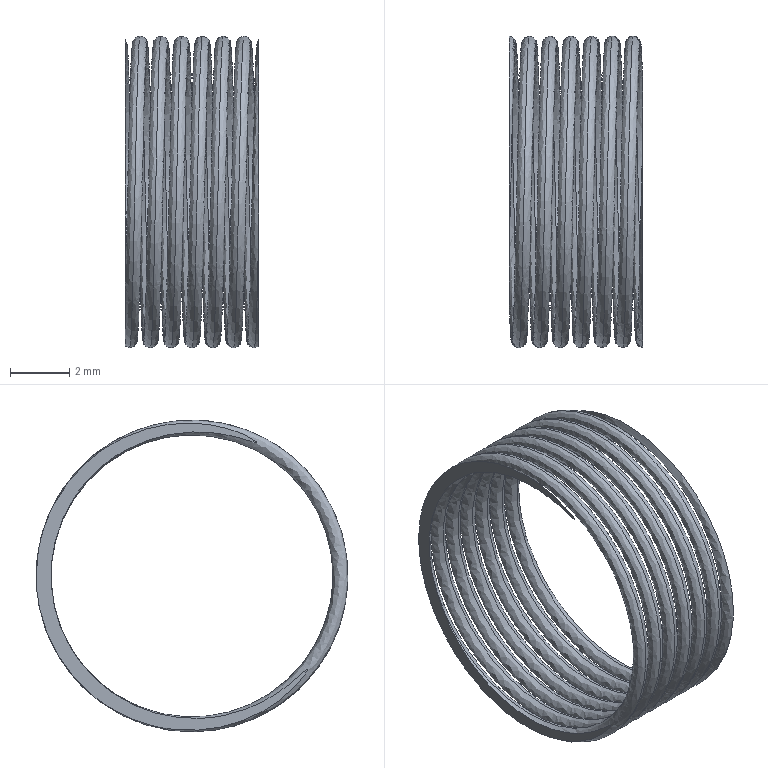Part | STEP file | 0246_015_WY10-15 | 1 solid | 4 faces | box 4.5 x 10.5 x 10.5 mm | volume 37.588 mm3 | spline 2 | plane 2